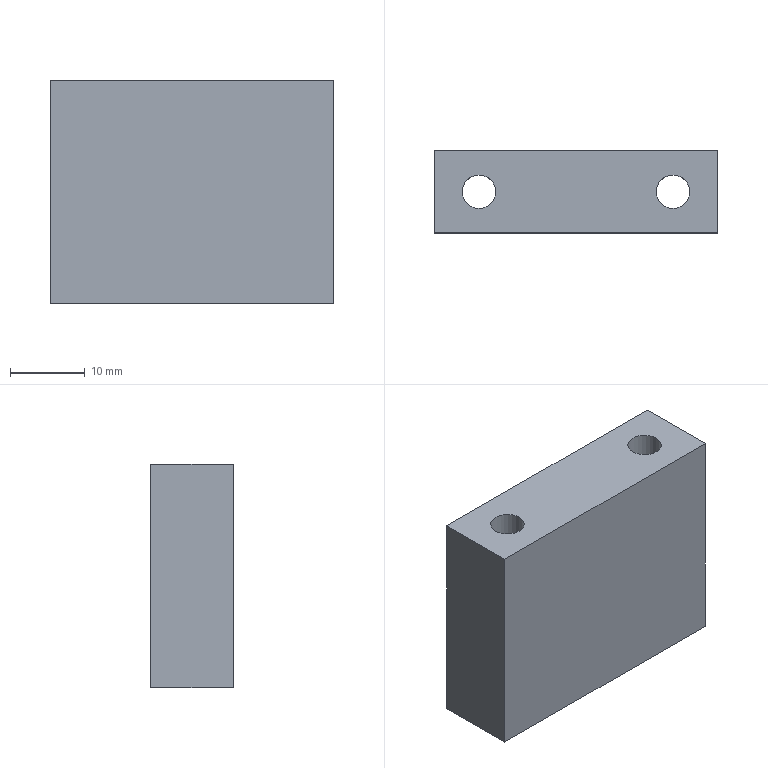Part | STEP file | 1 solid | 14 faces | box 38 x 11 x 30 mm | volume 9809 mm3 | plane 9 | cylinder 5 | commonest cylinder face diameters 8 x3 4.5 x2
STEP:
#1=CARTESIAN_POINT('',(0.,0.,0.));
#2=DIRECTION('',(0.,0.,1.));
#3=DIRECTION('',(1.,0.,0.));
#4=AXIS2_PLACEMENT_3D('',#1,#2,#3);
#5=CARTESIAN_POINT('',(-19.,5.5,-15.));
#6=VERTEX_POINT('',#5);
#7=CARTESIAN_POINT('',(19.,5.5,-15.));
#8=VERTEX_POINT('',#7);
#9=CARTESIAN_POINT('',(0.,5.5,-15.));
#10=DIRECTION('',(1.,0.,0.));
#11=VECTOR('',#10,1.);
#12=LINE('',#9,#11);
#13=CARTESIAN_POINT('',(0.,5.5,0.));
#14=DIRECTION('',(0.,-1.,0.));
#15=DIRECTION('',(0.,0.,-1.));
#16=AXIS2_PLACEMENT_3D('',#13,#14,#15);
#17=PLANE('',#16);
#18=CARTESIAN_POINT('',(15.,0.));
#19=DIRECTION('',(0.,1.));
#20=VECTOR('',#19,1.);
#21=LINE('',#18,#20);
#22=(GEOMETRIC_REPRESENTATION_CONTEXT(2)PARAMETRIC_REPRESENTATION_CONTEXT()REPRESENTATION_CONTEXT('',''));
#23=DEFINITIONAL_REPRESENTATION('',(#21),#22);
#24=PCURVE('',#17,#23);
#25=CARTESIAN_POINT('',(-19.,5.5,-15.));
#26=DIRECTION('',(0.,0.,1.));
#27=DIRECTION('',(1.,0.,0.));
#28=AXIS2_PLACEMENT_3D('',#25,#26,#27);
#29=PLANE('',#28);
#30=CARTESIAN_POINT('',(19.,0.));
#31=DIRECTION('',(1.,0.));
#32=VECTOR('',#31,1.);
#33=LINE('',#30,#32);
#34=(GEOMETRIC_REPRESENTATION_CONTEXT(2)PARAMETRIC_REPRESENTATION_CONTEXT()REPRESENTATION_CONTEXT('',''));
#35=DEFINITIONAL_REPRESENTATION('',(#33),#34);
#36=PCURVE('',#29,#35);
#37=SURFACE_CURVE('',#12,(#24,#36),.PCURVE_S1.);
#38=EDGE_CURVE('',#6,#8,#37,.T.);
#39=ORIENTED_EDGE('',*,*,#38,.F.);
#40=CARTESIAN_POINT('',(-19.,5.5,15.));
#41=VERTEX_POINT('',#40);
#42=CARTESIAN_POINT('',(-19.,5.5,0.));
#43=DIRECTION('',(0.,0.,-1.));
#44=VECTOR('',#43,1.);
#45=LINE('',#42,#44);
#46=CARTESIAN_POINT('',(0.,-19.));
#47=DIRECTION('',(1.,0.));
#48=VECTOR('',#47,1.);
#49=LINE('',#46,#48);
#50=(GEOMETRIC_REPRESENTATION_CONTEXT(2)PARAMETRIC_REPRESENTATION_CONTEXT()REPRESENTATION_CONTEXT('',''));
#51=DEFINITIONAL_REPRESENTATION('',(#49),#50);
#52=PCURVE('',#17,#51);
#53=CARTESIAN_POINT('',(-19.,5.5,15.));
#54=DIRECTION('',(1.,0.,0.));
#55=DIRECTION('',(0.,0.,-1.));
#56=AXIS2_PLACEMENT_3D('',#53,#54,#55);
#57=PLANE('',#56);
#58=CARTESIAN_POINT('',(15.,0.));
#59=DIRECTION('',(1.,0.));
#60=VECTOR('',#59,1.);
#61=LINE('',#58,#60);
#62=(GEOMETRIC_REPRESENTATION_CONTEXT(2)PARAMETRIC_REPRESENTATION_CONTEXT()REPRESENTATION_CONTEXT('',''));
#63=DEFINITIONAL_REPRESENTATION('',(#61),#62);
#64=PCURVE('',#57,#63);
#65=SURFACE_CURVE('',#45,(#52,#64),.PCURVE_S1.);
#66=EDGE_CURVE('',#41,#6,#65,.T.);
#67=ORIENTED_EDGE('',*,*,#66,.F.);
#68=CARTESIAN_POINT('',(19.,5.5,15.));
#69=VERTEX_POINT('',#68);
#70=CARTESIAN_POINT('',(0.,5.5,15.));
#71=DIRECTION('',(-1.,0.,0.));
#72=VECTOR('',#71,1.);
#73=LINE('',#70,#72);
#74=CARTESIAN_POINT('',(-15.,0.));
#75=DIRECTION('',(0.,-1.));
#76=VECTOR('',#75,1.);
#77=LINE('',#74,#76);
#78=(GEOMETRIC_REPRESENTATION_CONTEXT(2)PARAMETRIC_REPRESENTATION_CONTEXT()REPRESENTATION_CONTEXT('',''));
#79=DEFINITIONAL_REPRESENTATION('',(#77),#78);
#80=PCURVE('',#17,#79);
#81=CARTESIAN_POINT('',(-19.,5.5,15.));
#82=DIRECTION('',(0.,0.,-1.));
#83=DIRECTION('',(-1.,0.,0.));
#84=AXIS2_PLACEMENT_3D('',#81,#82,#83);
#85=PLANE('',#84);
#86=CARTESIAN_POINT('',(-19.,0.));
#87=DIRECTION('',(1.,0.));
#88=VECTOR('',#87,1.);
#89=LINE('',#86,#88);
#90=(GEOMETRIC_REPRESENTATION_CONTEXT(2)PARAMETRIC_REPRESENTATION_CONTEXT()REPRESENTATION_CONTEXT('',''));
#91=DEFINITIONAL_REPRESENTATION('',(#89),#90);
#92=PCURVE('',#85,#91);
#93=SURFACE_CURVE('',#73,(#80,#92),.PCURVE_S1.);
#94=EDGE_CURVE('',#69,#41,#93,.T.);
#95=ORIENTED_EDGE('',*,*,#94,.F.);
#96=CARTESIAN_POINT('',(19.,5.5,0.));
#97=DIRECTION('',(0.,0.,1.));
#98=VECTOR('',#97,1.);
#99=LINE('',#96,#98);
#100=CARTESIAN_POINT('',(0.,19.));
#101=DIRECTION('',(-1.,0.));
#102=VECTOR('',#101,1.);
#103=LINE('',#100,#102);
#104=(GEOMETRIC_REPRESENTATION_CONTEXT(2)PARAMETRIC_REPRESENTATION_CONTEXT()REPRESENTATION_CONTEXT('',''));
#105=DEFINITIONAL_REPRESENTATION('',(#103),#104);
#106=PCURVE('',#17,#105);
#107=CARTESIAN_POINT('',(19.,5.5,15.));
#108=DIRECTION('',(-1.,0.,0.));
#109=DIRECTION('',(0.,0.,1.));
#110=AXIS2_PLACEMENT_3D('',#107,#108,#109);
#111=PLANE('',#110);
#112=CARTESIAN_POINT('',(-15.,0.));
#113=DIRECTION('',(1.,0.));
#114=VECTOR('',#113,1.);
#115=LINE('',#112,#114);
#116=(GEOMETRIC_REPRESENTATION_CONTEXT(2)PARAMETRIC_REPRESENTATION_CONTEXT()REPRESENTATION_CONTEXT('',''));
#117=DEFINITIONAL_REPRESENTATION('',(#115),#116);
#118=PCURVE('',#111,#117);
#119=SURFACE_CURVE('',#99,(#106,#118),.PCURVE_S1.);
#120=EDGE_CURVE('',#8,#69,#119,.T.);
#121=ORIENTED_EDGE('',*,*,#120,.F.);
#122=EDGE_LOOP('',(#39,#67,#95,#121));
#123=FACE_BOUND('',#122,.T.);
#124=ADVANCED_FACE('',(#123),#17,.F.);
#125=CARTESIAN_POINT('',(19.,-5.5,-15.));
#126=VERTEX_POINT('',#125);
#127=CARTESIAN_POINT('',(19.,5.5,-15.));
#128=DIRECTION('',(0.,-1.,0.));
#129=VECTOR('',#128,1.);
#130=LINE('',#127,#129);
#131=CARTESIAN_POINT('',(-30.,0.));
#132=DIRECTION('',(0.,-1.));
#133=VECTOR('',#132,1.);
#134=LINE('',#131,#133);
#135=(GEOMETRIC_REPRESENTATION_CONTEXT(2)PARAMETRIC_REPRESENTATION_CONTEXT()REPRESENTATION_CONTEXT('',''));
#136=DEFINITIONAL_REPRESENTATION('',(#134),#135);
#137=PCURVE('',#111,#136);
#138=CARTESIAN_POINT('',(38.,0.));
#139=DIRECTION('',(0.,-1.));
#140=VECTOR('',#139,1.);
#141=LINE('',#138,#140);
#142=(GEOMETRIC_REPRESENTATION_CONTEXT(2)PARAMETRIC_REPRESENTATION_CONTEXT()REPRESENTATION_CONTEXT('',''));
#143=DEFINITIONAL_REPRESENTATION('',(#141),#142);
#144=PCURVE('',#29,#143);
#145=SURFACE_CURVE('',#130,(#137,#144),.PCURVE_S1.);
#146=EDGE_CURVE('',#8,#126,#145,.T.);
#147=ORIENTED_EDGE('',*,*,#146,.F.);
#148=ORIENTED_EDGE('',*,*,#120,.T.);
#149=CARTESIAN_POINT('',(19.,-5.5,15.));
#150=VERTEX_POINT('',#149);
#151=CARTESIAN_POINT('',(19.,5.5,15.));
#152=DIRECTION('',(0.,1.,0.));
#153=VECTOR('',#152,1.);
#154=LINE('',#151,#153);
#155=CARTESIAN_POINT('',(0.,0.));
#156=DIRECTION('',(0.,1.));
#157=VECTOR('',#156,1.);
#158=LINE('',#155,#157);
#159=(GEOMETRIC_REPRESENTATION_CONTEXT(2)PARAMETRIC_REPRESENTATION_CONTEXT()REPRESENTATION_CONTEXT('',''));
#160=DEFINITIONAL_REPRESENTATION('',(#158),#159);
#161=PCURVE('',#111,#160);
#162=CARTESIAN_POINT('',(-38.,0.));
#163=DIRECTION('',(0.,1.));
#164=VECTOR('',#163,1.);
#165=LINE('',#162,#164);
#166=(GEOMETRIC_REPRESENTATION_CONTEXT(2)PARAMETRIC_REPRESENTATION_CONTEXT()REPRESENTATION_CONTEXT('',''));
#167=DEFINITIONAL_REPRESENTATION('',(#165),#166);
#168=PCURVE('',#85,#167);
#169=SURFACE_CURVE('',#154,(#161,#168),.PCURVE_S1.);
#170=EDGE_CURVE('',#150,#69,#169,.T.);
#171=ORIENTED_EDGE('',*,*,#170,.F.);
#172=CARTESIAN_POINT('',(19.,-5.5,15.));
#173=DIRECTION('',(0.,0.,1.));
#174=VECTOR('',#173,1.);
#175=LINE('',#172,#174);
#176=CARTESIAN_POINT('',(0.,-11.));
#177=DIRECTION('',(1.,0.));
#178=VECTOR('',#177,1.);
#179=LINE('',#176,#178);
#180=(GEOMETRIC_REPRESENTATION_CONTEXT(2)PARAMETRIC_REPRESENTATION_CONTEXT()REPRESENTATION_CONTEXT('',''));
#181=DEFINITIONAL_REPRESENTATION('',(#179),#180);
#182=PCURVE('',#111,#181);
#183=CARTESIAN_POINT('',(0.,-5.5,0.));
#184=DIRECTION('',(0.,-1.,0.));
#185=DIRECTION('',(0.,0.,-1.));
#186=AXIS2_PLACEMENT_3D('',#183,#184,#185);
#187=PLANE('',#186);
#188=CARTESIAN_POINT('',(-15.,19.));
#189=DIRECTION('',(-1.,0.));
#190=VECTOR('',#189,1.);
#191=LINE('',#188,#190);
#192=(GEOMETRIC_REPRESENTATION_CONTEXT(2)PARAMETRIC_REPRESENTATION_CONTEXT()REPRESENTATION_CONTEXT('',''));
#193=DEFINITIONAL_REPRESENTATION('',(#191),#192);
#194=PCURVE('',#187,#193);
#195=SURFACE_CURVE('',#175,(#182,#194),.PCURVE_S1.);
#196=EDGE_CURVE('',#126,#150,#195,.T.);
#197=ORIENTED_EDGE('',*,*,#196,.F.);
#198=EDGE_LOOP('',(#147,#148,#171,#197));
#199=FACE_BOUND('',#198,.T.);
#200=ADVANCED_FACE('',(#199),#111,.F.);
#201=CARTESIAN_POINT('',(-17.,0.,-15.));
#202=VERTEX_POINT('',#201);
#203=CARTESIAN_POINT('',(-13.,0.,-15.));
#204=DIRECTION('',(0.,0.,-1.));
#205=DIRECTION('',(-1.,0.,0.));
#206=AXIS2_PLACEMENT_3D('',#203,#204,#205);
#207=CIRCLE('',#206,4.);
#208=CARTESIAN_POINT('',(2.,-5.5));
#209=CARTESIAN_POINT('',(2.,1.428));
#210=CARTESIAN_POINT('',(8.,-2.036));
#211=CARTESIAN_POINT('',(14.,-5.5));
#212=CARTESIAN_POINT('',(8.,-8.964));
#213=CARTESIAN_POINT('',(2.,-12.428));
#214=CARTESIAN_POINT('',(2.,-5.5));
#215=(BOUNDED_CURVE()B_SPLINE_CURVE(2,(#208,#209,#210,#211,#212,#213,#214),.UNSPECIFIED.,.T.,.F.)B_SPLINE_CURVE_WITH_KNOTS((1,2,2,2,2,1),(-2.094,0.,2.094,4.189,6.283,8.378),.UNSPECIFIED.)CURVE()GEOMETRIC_REPRESENTATION_ITEM()RATIONAL_B_SPLINE_CURVE((1.,0.5,1.,0.5,1.,0.5,1.))REPRESENTATION_ITEM(''));
#216=(GEOMETRIC_REPRESENTATION_CONTEXT(2)PARAMETRIC_REPRESENTATION_CONTEXT()REPRESENTATION_CONTEXT('',''));
#217=DEFINITIONAL_REPRESENTATION('',(#215),#216);
#218=PCURVE('',#29,#217);
#219=CARTESIAN_POINT('',(-13.,0.,-15.));
#220=DIRECTION('',(0.,0.,-1.));
#221=DIRECTION('',(-1.,0.,0.));
#222=AXIS2_PLACEMENT_3D('',#219,#220,#221);
#223=CYLINDRICAL_SURFACE('',#222,4.);
#224=CARTESIAN_POINT('',(0.,0.));
#225=DIRECTION('',(1.,0.));
#226=VECTOR('',#225,1.);
#227=LINE('',#224,#226);
#228=(GEOMETRIC_REPRESENTATION_CONTEXT(2)PARAMETRIC_REPRESENTATION_CONTEXT()REPRESENTATION_CONTEXT('',''));
#229=DEFINITIONAL_REPRESENTATION('',(#227),#228);
#230=PCURVE('',#223,#229);
#231=SURFACE_CURVE('',#207,(#218,#230),.PCURVE_S1.);
#232=EDGE_CURVE('',#202,#202,#231,.T.);
#233=ORIENTED_EDGE('',*,*,#232,.F.);
#234=EDGE_LOOP('',(#233));
#235=FACE_BOUND('',#234,.T.);
#236=CARTESIAN_POINT('',(9.,0.,-15.));
#237=VERTEX_POINT('',#236);
#238=CARTESIAN_POINT('',(13.,0.,-15.));
#239=DIRECTION('',(0.,0.,-1.));
#240=DIRECTION('',(-1.,0.,0.));
#241=AXIS2_PLACEMENT_3D('',#238,#239,#240);
#242=CIRCLE('',#241,4.);
#243=CARTESIAN_POINT('',(28.,-5.5));
#244=CARTESIAN_POINT('',(28.,1.428));
#245=CARTESIAN_POINT('',(34.,-2.036));
#246=CARTESIAN_POINT('',(40.,-5.5));
#247=CARTESIAN_POINT('',(34.,-8.964));
#248=CARTESIAN_POINT('',(28.,-12.428));
#249=CARTESIAN_POINT('',(28.,-5.5));
#250=(BOUNDED_CURVE()B_SPLINE_CURVE(2,(#243,#244,#245,#246,#247,#248,#249),.UNSPECIFIED.,.T.,.F.)B_SPLINE_CURVE_WITH_KNOTS((1,2,2,2,2,1),(-2.094,0.,2.094,4.189,6.283,8.378),.UNSPECIFIED.)CURVE()GEOMETRIC_REPRESENTATION_ITEM()RATIONAL_B_SPLINE_CURVE((1.,0.5,1.,0.5,1.,0.5,1.))REPRESENTATION_ITEM(''));
#251=(GEOMETRIC_REPRESENTATION_CONTEXT(2)PARAMETRIC_REPRESENTATION_CONTEXT()REPRESENTATION_CONTEXT('',''));
#252=DEFINITIONAL_REPRESENTATION('',(#250),#251);
#253=PCURVE('',#29,#252);
#254=CARTESIAN_POINT('',(13.,0.,-15.));
#255=DIRECTION('',(0.,0.,-1.));
#256=DIRECTION('',(-1.,0.,0.));
#257=AXIS2_PLACEMENT_3D('',#254,#255,#256);
#258=CYLINDRICAL_SURFACE('',#257,4.);
#259=CARTESIAN_POINT('',(0.,0.));
#260=DIRECTION('',(1.,0.));
#261=VECTOR('',#260,1.);
#262=LINE('',#259,#261);
#263=(GEOMETRIC_REPRESENTATION_CONTEXT(2)PARAMETRIC_REPRESENTATION_CONTEXT()REPRESENTATION_CONTEXT('',''));
#264=DEFINITIONAL_REPRESENTATION('',(#262),#263);
#265=PCURVE('',#258,#264);
#266=SURFACE_CURVE('',#242,(#253,#265),.PCURVE_S1.);
#267=EDGE_CURVE('',#237,#237,#266,.T.);
#268=ORIENTED_EDGE('',*,*,#267,.F.);
#269=EDGE_LOOP('',(#268));
#270=FACE_BOUND('',#269,.T.);
#271=CARTESIAN_POINT('',(-4.,0.,-15.));
#272=VERTEX_POINT('',#271);
#273=CARTESIAN_POINT('',(0.,0.,-15.));
#274=DIRECTION('',(0.,0.,-1.));
#275=DIRECTION('',(-1.,0.,0.));
#276=AXIS2_PLACEMENT_3D('',#273,#274,#275);
#277=CIRCLE('',#276,4.);
#278=CARTESIAN_POINT('',(15.,-5.5));
#279=CARTESIAN_POINT('',(15.,1.428));
#280=CARTESIAN_POINT('',(21.,-2.036));
#281=CARTESIAN_POINT('',(27.,-5.5));
#282=CARTESIAN_POINT('',(21.,-8.964));
#283=CARTESIAN_POINT('',(15.,-12.428));
#284=CARTESIAN_POINT('',(15.,-5.5));
#285=(BOUNDED_CURVE()B_SPLINE_CURVE(2,(#278,#279,#280,#281,#282,#283,#284),.UNSPECIFIED.,.T.,.F.)B_SPLINE_CURVE_WITH_KNOTS((1,2,2,2,2,1),(-2.094,0.,2.094,4.189,6.283,8.378),.UNSPECIFIED.)CURVE()GEOMETRIC_REPRESENTATION_ITEM()RATIONAL_B_SPLINE_CURVE((1.,0.5,1.,0.5,1.,0.5,1.))REPRESENTATION_ITEM(''));
#286=(GEOMETRIC_REPRESENTATION_CONTEXT(2)PARAMETRIC_REPRESENTATION_CONTEXT()REPRESENTATION_CONTEXT('',''));
#287=DEFINITIONAL_REPRESENTATION('',(#285),#286);
#288=PCURVE('',#29,#287);
#289=CARTESIAN_POINT('',(0.,0.,-7.));
#290=DIRECTION('',(0.,0.,-1.));
#291=DIRECTION('',(-1.,0.,0.));
#292=AXIS2_PLACEMENT_3D('',#289,#290,#291);
#293=CYLINDRICAL_SURFACE('',#292,4.);
#294=CARTESIAN_POINT('',(0.,8.));
#295=DIRECTION('',(1.,0.));
#296=VECTOR('',#295,1.);
#297=LINE('',#294,#296);
#298=(GEOMETRIC_REPRESENTATION_CONTEXT(2)PARAMETRIC_REPRESENTATION_CONTEXT()REPRESENTATION_CONTEXT('',''));
#299=DEFINITIONAL_REPRESENTATION('',(#297),#298);
#300=PCURVE('',#293,#299);
#301=SURFACE_CURVE('',#277,(#288,#300),.PCURVE_S1.);
#302=EDGE_CURVE('',#272,#272,#301,.T.);
#303=ORIENTED_EDGE('',*,*,#302,.F.);
#304=EDGE_LOOP('',(#303));
#305=FACE_BOUND('',#304,.T.);
#306=CARTESIAN_POINT('',(-19.,-5.5,-15.));
#307=VERTEX_POINT('',#306);
#308=CARTESIAN_POINT('',(-19.,5.5,-15.));
#309=DIRECTION('',(0.,-1.,0.));
#310=VECTOR('',#309,1.);
#311=LINE('',#308,#310);
#312=CARTESIAN_POINT('',(0.,0.));
#313=DIRECTION('',(0.,-1.));
#314=VECTOR('',#313,1.);
#315=LINE('',#312,#314);
#316=(GEOMETRIC_REPRESENTATION_CONTEXT(2)PARAMETRIC_REPRESENTATION_CONTEXT()REPRESENTATION_CONTEXT('',''));
#317=DEFINITIONAL_REPRESENTATION('',(#315),#316);
#318=PCURVE('',#29,#317);
#319=CARTESIAN_POINT('',(30.,0.));
#320=DIRECTION('',(0.,-1.));
#321=VECTOR('',#320,1.);
#322=LINE('',#319,#321);
#323=(GEOMETRIC_REPRESENTATION_CONTEXT(2)PARAMETRIC_REPRESENTATION_CONTEXT()REPRESENTATION_CONTEXT('',''));
#324=DEFINITIONAL_REPRESENTATION('',(#322),#323);
#325=PCURVE('',#57,#324);
#326=SURFACE_CURVE('',#311,(#318,#325),.PCURVE_S1.);
#327=EDGE_CURVE('',#6,#307,#326,.T.);
#328=ORIENTED_EDGE('',*,*,#327,.F.);
#329=ORIENTED_EDGE('',*,*,#38,.T.);
#330=ORIENTED_EDGE('',*,*,#146,.T.);
#331=CARTESIAN_POINT('',(-19.,-5.5,-15.));
#332=DIRECTION('',(1.,0.,0.));
#333=VECTOR('',#332,1.);
#334=LINE('',#331,#333);
#335=CARTESIAN_POINT('',(0.,-11.));
#336=DIRECTION('',(1.,0.));
#337=VECTOR('',#336,1.);
#338=LINE('',#335,#337);
#339=(GEOMETRIC_REPRESENTATION_CONTEXT(2)PARAMETRIC_REPRESENTATION_CONTEXT()REPRESENTATION_CONTEXT('',''));
#340=DEFINITIONAL_REPRESENTATION('',(#338),#339);
#341=PCURVE('',#29,#340);
#342=CARTESIAN_POINT('',(15.,-19.));
#343=DIRECTION('',(0.,1.));
#344=VECTOR('',#343,1.);
#345=LINE('',#342,#344);
#346=(GEOMETRIC_REPRESENTATION_CONTEXT(2)PARAMETRIC_REPRESENTATION_CONTEXT()REPRESENTATION_CONTEXT('',''));
#347=DEFINITIONAL_REPRESENTATION('',(#345),#346);
#348=PCURVE('',#187,#347);
#349=SURFACE_CURVE('',#334,(#341,#348),.PCURVE_S1.);
#350=EDGE_CURVE('',#307,#126,#349,.T.);
#351=ORIENTED_EDGE('',*,*,#350,.F.);
#352=EDGE_LOOP('',(#328,#329,#330,#351));
#353=FACE_BOUND('',#352,.T.);
#354=ADVANCED_FACE('',(#235,#270,#305,#353),#29,.F.);
#355=CARTESIAN_POINT('',(-19.,-5.5,15.));
#356=VERTEX_POINT('',#355);
#357=CARTESIAN_POINT('',(-19.,5.5,15.));
#358=DIRECTION('',(0.,-1.,0.));
#359=VECTOR('',#358,1.);
#360=LINE('',#357,#359);
#361=CARTESIAN_POINT('',(0.,0.));
#362=DIRECTION('',(0.,-1.));
#363=VECTOR('',#362,1.);
#364=LINE('',#361,#363);
#365=(GEOMETRIC_REPRESENTATION_CONTEXT(2)PARAMETRIC_REPRESENTATION_CONTEXT()REPRESENTATION_CONTEXT('',''));
#366=DEFINITIONAL_REPRESENTATION('',(#364),#365);
#367=PCURVE('',#57,#366);
#368=CARTESIAN_POINT('',(0.,0.));
#369=DIRECTION('',(0.,-1.));
#370=VECTOR('',#369,1.);
#371=LINE('',#368,#370);
#372=(GEOMETRIC_REPRESENTATION_CONTEXT(2)PARAMETRIC_REPRESENTATION_CONTEXT()REPRESENTATION_CONTEXT('',''));
#373=DEFINITIONAL_REPRESENTATION('',(#371),#372);
#374=PCURVE('',#85,#373);
#375=SURFACE_CURVE('',#360,(#367,#374),.PCURVE_S1.);
#376=EDGE_CURVE('',#41,#356,#375,.T.);
#377=ORIENTED_EDGE('',*,*,#376,.F.);
#378=ORIENTED_EDGE('',*,*,#66,.T.);
#379=ORIENTED_EDGE('',*,*,#327,.T.);
#380=CARTESIAN_POINT('',(-19.,-5.5,15.));
#381=DIRECTION('',(0.,0.,-1.));
#382=VECTOR('',#381,1.);
#383=LINE('',#380,#382);
#384=CARTESIAN_POINT('',(0.,-11.));
#385=DIRECTION('',(1.,0.));
#386=VECTOR('',#385,1.);
#387=LINE('',#384,#386);
#388=(GEOMETRIC_REPRESENTATION_CONTEXT(2)PARAMETRIC_REPRESENTATION_CONTEXT()REPRESENTATION_CONTEXT('',''));
#389=DEFINITIONAL_REPRESENTATION('',(#387),#388);
#390=PCURVE('',#57,#389);
#391=CARTESIAN_POINT('',(-15.,-19.));
#392=DIRECTION('',(1.,0.));
#393=VECTOR('',#392,1.);
#394=LINE('',#391,#393);
#395=(GEOMETRIC_REPRESENTATION_CONTEXT(2)PARAMETRIC_REPRESENTATION_CONTEXT()REPRESENTATION_CONTEXT('',''));
#396=DEFINITIONAL_REPRESENTATION('',(#394),#395);
#397=PCURVE('',#187,#396);
#398=SURFACE_CURVE('',#383,(#390,#397),.PCURVE_S1.);
#399=EDGE_CURVE('',#356,#307,#398,.T.);
#400=ORIENTED_EDGE('',*,*,#399,.F.);
#401=EDGE_LOOP('',(#377,#378,#379,#400));
#402=FACE_BOUND('',#401,.T.);
#403=ADVANCED_FACE('',(#402),#57,.F.);
#404=CARTESIAN_POINT('',(-15.25,0.,15.));
#405=VERTEX_POINT('',#404);
#406=CARTESIAN_POINT('',(-13.,0.,15.));
#407=DIRECTION('',(0.,0.,1.));
#408=DIRECTION('',(-1.,0.,0.));
#409=AXIS2_PLACEMENT_3D('',#406,#407,#408);
#410=CIRCLE('',#409,2.25);
#411=CARTESIAN_POINT('',(-3.75,-5.5));
#412=CARTESIAN_POINT('',(-3.75,-9.397));
#413=CARTESIAN_POINT('',(-7.125,-7.449));
#414=CARTESIAN_POINT('',(-10.5,-5.5));
#415=CARTESIAN_POINT('',(-7.125,-3.551));
#416=CARTESIAN_POINT('',(-3.75,-1.603));
#417=CARTESIAN_POINT('',(-3.75,-5.5));
#418=(BOUNDED_CURVE()B_SPLINE_CURVE(2,(#411,#412,#413,#414,#415,#416,#417),.UNSPECIFIED.,.T.,.F.)B_SPLINE_CURVE_WITH_KNOTS((1,2,2,2,2,1),(-2.094,0.,2.094,4.189,6.283,8.378),.UNSPECIFIED.)CURVE()GEOMETRIC_REPRESENTATION_ITEM()RATIONAL_B_SPLINE_CURVE((1.,0.5,1.,0.5,1.,0.5,1.))REPRESENTATION_ITEM(''));
#419=(GEOMETRIC_REPRESENTATION_CONTEXT(2)PARAMETRIC_REPRESENTATION_CONTEXT()REPRESENTATION_CONTEXT('',''));
#420=DEFINITIONAL_REPRESENTATION('',(#418),#419);
#421=PCURVE('',#85,#420);
#422=CARTESIAN_POINT('',(-13.,0.,-15.));
#423=DIRECTION('',(0.,0.,-1.));
#424=DIRECTION('',(-1.,0.,0.));
#425=AXIS2_PLACEMENT_3D('',#422,#423,#424);
#426=CYLINDRICAL_SURFACE('',#425,2.25);
#427=CARTESIAN_POINT('',(6.283,-30.));
#428=DIRECTION('',(-1.,0.));
#429=VECTOR('',#428,1.);
#430=LINE('',#427,#429);
#431=(GEOMETRIC_REPRESENTATION_CONTEXT(2)PARAMETRIC_REPRESENTATION_CONTEXT()REPRESENTATION_CONTEXT('',''));
#432=DEFINITIONAL_REPRESENTATION('',(#430),#431);
#433=PCURVE('',#426,#432);
#434=SURFACE_CURVE('',#410,(#421,#433),.PCURVE_S1.);
#435=EDGE_CURVE('',#405,#405,#434,.T.);
#436=ORIENTED_EDGE('',*,*,#435,.F.);
#437=EDGE_LOOP('',(#436));
#438=FACE_BOUND('',#437,.T.);
#439=CARTESIAN_POINT('',(10.75,0.,15.));
#440=VERTEX_POINT('',#439);
#441=CARTESIAN_POINT('',(13.,0.,15.));
#442=DIRECTION('',(0.,0.,1.));
#443=DIRECTION('',(-1.,0.,0.));
#444=AXIS2_PLACEMENT_3D('',#441,#442,#443);
#445=CIRCLE('',#444,2.25);
#446=CARTESIAN_POINT('',(-29.75,-5.5));
#447=CARTESIAN_POINT('',(-29.75,-9.397));
#448=CARTESIAN_POINT('',(-33.125,-7.449));
#449=CARTESIAN_POINT('',(-36.5,-5.5));
#450=CARTESIAN_POINT('',(-33.125,-3.551));
#451=CARTESIAN_POINT('',(-29.75,-1.603));
#452=CARTESIAN_POINT('',(-29.75,-5.5));
#453=(BOUNDED_CURVE()B_SPLINE_CURVE(2,(#446,#447,#448,#449,#450,#451,#452),.UNSPECIFIED.,.T.,.F.)B_SPLINE_CURVE_WITH_KNOTS((1,2,2,2,2,1),(-2.094,0.,2.094,4.189,6.283,8.378),.UNSPECIFIED.)CURVE()GEOMETRIC_REPRESENTATION_ITEM()RATIONAL_B_SPLINE_CURVE((1.,0.5,1.,0.5,1.,0.5,1.))REPRESENTATION_ITEM(''));
#454=(GEOMETRIC_REPRESENTATION_CONTEXT(2)PARAMETRIC_REPRESENTATION_CONTEXT()REPRESENTATION_CONTEXT('',''));
#455=DEFINITIONAL_REPRESENTATION('',(#453),#454);
#456=PCURVE('',#85,#455);
#457=CARTESIAN_POINT('',(13.,0.,-15.));
#458=DIRECTION('',(0.,0.,-1.));
#459=DIRECTION('',(-1.,0.,0.));
#460=AXIS2_PLACEMENT_3D('',#457,#458,#459);
#461=CYLINDRICAL_SURFACE('',#460,2.25);
#462=CARTESIAN_POINT('',(6.283,-30.));
#463=DIRECTION('',(-1.,0.));
#464=VECTOR('',#463,1.);
#465=LINE('',#462,#464);
#466=(GEOMETRIC_REPRESENTATION_CONTEXT(2)PARAMETRIC_REPRESENTATION_CONTEXT()REPRESENTATION_CONTEXT('',''));
#467=DEFINITIONAL_REPRESENTATION('',(#465),#466);
#468=PCURVE('',#461,#467);
#469=SURFACE_CURVE('',#445,(#456,#468),.PCURVE_S1.);
#470=EDGE_CURVE('',#440,#440,#469,.T.);
#471=ORIENTED_EDGE('',*,*,#470,.F.);
#472=EDGE_LOOP('',(#471));
#473=FACE_BOUND('',#472,.T.);
#474=ORIENTED_EDGE('',*,*,#170,.T.);
#475=ORIENTED_EDGE('',*,*,#94,.T.);
#476=ORIENTED_EDGE('',*,*,#376,.T.);
#477=CARTESIAN_POINT('',(-19.,-5.5,15.));
#478=DIRECTION('',(-1.,0.,0.));
#479=VECTOR('',#478,1.);
#480=LINE('',#477,#479);
#481=CARTESIAN_POINT('',(0.,-11.));
#482=DIRECTION('',(1.,0.));
#483=VECTOR('',#482,1.);
#484=LINE('',#481,#483);
#485=(GEOMETRIC_REPRESENTATION_CONTEXT(2)PARAMETRIC_REPRESENTATION_CONTEXT()REPRESENTATION_CONTEXT('',''));
#486=DEFINITIONAL_REPRESENTATION('',(#484),#485);
#487=PCURVE('',#85,#486);
#488=CARTESIAN_POINT('',(-15.,-19.));
#489=DIRECTION('',(0.,-1.));
#490=VECTOR('',#489,1.);
#491=LINE('',#488,#490);
#492=(GEOMETRIC_REPRESENTATION_CONTEXT(2)PARAMETRIC_REPRESENTATION_CONTEXT()REPRESENTATION_CONTEXT('',''));
#493=DEFINITIONAL_REPRESENTATION('',(#491),#492);
#494=PCURVE('',#187,#493);
#495=SURFACE_CURVE('',#480,(#487,#494),.PCURVE_S1.);
#496=EDGE_CURVE('',#150,#356,#495,.T.);
#497=ORIENTED_EDGE('',*,*,#496,.F.);
#498=EDGE_LOOP('',(#474,#475,#476,#497));
#499=FACE_BOUND('',#498,.T.);
#500=ADVANCED_FACE('',(#438,#473,#499),#85,.F.);
#501=ORIENTED_EDGE('',*,*,#399,.T.);
#502=ORIENTED_EDGE('',*,*,#350,.T.);
#503=ORIENTED_EDGE('',*,*,#196,.T.);
#504=ORIENTED_EDGE('',*,*,#496,.T.);
#505=EDGE_LOOP('',(#501,#502,#503,#504));
#506=FACE_BOUND('',#505,.T.);
#507=ADVANCED_FACE('',(#506),#187,.T.);
#508=CARTESIAN_POINT('',(-17.,0.,5.));
#509=VERTEX_POINT('',#508);
#510=CARTESIAN_POINT('',(-13.,0.,5.));
#511=DIRECTION('',(0.,0.,-1.));
#512=DIRECTION('',(-1.,0.,0.));
#513=AXIS2_PLACEMENT_3D('',#510,#511,#512);
#514=CIRCLE('',#513,4.);
#515=CARTESIAN_POINT('',(0.,-20.));
#516=DIRECTION('',(1.,0.));
#517=VECTOR('',#516,1.);
#518=LINE('',#515,#517);
#519=(GEOMETRIC_REPRESENTATION_CONTEXT(2)PARAMETRIC_REPRESENTATION_CONTEXT()REPRESENTATION_CONTEXT('',''));
#520=DEFINITIONAL_REPRESENTATION('',(#518),#519);
#521=PCURVE('',#223,#520);
#522=CARTESIAN_POINT('',(-10.75,0.,5.));
#523=DIRECTION('',(0.,0.,1.));
#524=DIRECTION('',(1.,0.,0.));
#525=AXIS2_PLACEMENT_3D('',#522,#523,#524);
#526=PLANE('',#525);
#527=CARTESIAN_POINT('',(-6.25,0.));
#528=CARTESIAN_POINT('',(-6.25,6.928));
#529=CARTESIAN_POINT('',(-0.25,3.464));
#530=CARTESIAN_POINT('',(5.75,0.));
#531=CARTESIAN_POINT('',(-0.25,-3.464));
#532=CARTESIAN_POINT('',(-6.25,-6.928));
#533=CARTESIAN_POINT('',(-6.25,0.));
#534=(BOUNDED_CURVE()B_SPLINE_CURVE(2,(#527,#528,#529,#530,#531,#532,#533),.UNSPECIFIED.,.T.,.F.)B_SPLINE_CURVE_WITH_KNOTS((1,2,2,2,2,1),(-2.094,0.,2.094,4.189,6.283,8.378),.UNSPECIFIED.)CURVE()GEOMETRIC_REPRESENTATION_ITEM()RATIONAL_B_SPLINE_CURVE((1.,0.5,1.,0.5,1.,0.5,1.))REPRESENTATION_ITEM(''));
#535=(GEOMETRIC_REPRESENTATION_CONTEXT(2)PARAMETRIC_REPRESENTATION_CONTEXT()REPRESENTATION_CONTEXT('',''));
#536=DEFINITIONAL_REPRESENTATION('',(#534),#535);
#537=PCURVE('',#526,#536);
#538=SURFACE_CURVE('',#514,(#521,#537),.PCURVE_S1.);
#539=EDGE_CURVE('',#509,#509,#538,.T.);
#540=ORIENTED_EDGE('',*,*,#539,.T.);
#541=CARTESIAN_POINT('',(-17.,0.,5.));
#542=CARTESIAN_POINT('',(-17.,0.,-15.));
#543=B_SPLINE_CURVE_WITH_KNOTS('',1,(#541,#542),.UNSPECIFIED.,.F.,.F.,(2,2),(-20.,0.),.PIECEWISE_BEZIER_KNOTS.);
#544=CARTESIAN_POINT('',(6.283,0.));
#545=DIRECTION('',(0.,1.));
#546=VECTOR('',#545,1.);
#547=LINE('',#544,#546);
#548=(GEOMETRIC_REPRESENTATION_CONTEXT(2)PARAMETRIC_REPRESENTATION_CONTEXT()REPRESENTATION_CONTEXT('',''));
#549=DEFINITIONAL_REPRESENTATION('',(#547),#548);
#550=PCURVE('',#223,#549);
#551=CARTESIAN_POINT('',(0.,0.));
#552=DIRECTION('',(0.,1.));
#553=VECTOR('',#552,1.);
#554=LINE('',#551,#553);
#555=(GEOMETRIC_REPRESENTATION_CONTEXT(2)PARAMETRIC_REPRESENTATION_CONTEXT()REPRESENTATION_CONTEXT('',''));
#556=DEFINITIONAL_REPRESENTATION('',(#554),#555);
#557=PCURVE('',#223,#556);
#558=SEAM_CURVE('',#543,(#550,#557),.PCURVE_S1.);
#559=EDGE_CURVE('',#509,#202,#558,.T.);
#560=ORIENTED_EDGE('',*,*,#559,.T.);
#561=ORIENTED_EDGE('',*,*,#232,.F.);
#562=ORIENTED_EDGE('',*,*,#559,.F.);
#563=EDGE_LOOP('',(#540,#560,#561,#562));
#564=FACE_BOUND('',#563,.F.);
#565=ADVANCED_FACE('',(#564),#223,.F.);
#566=CARTESIAN_POINT('',(9.,0.,5.));
#567=VERTEX_POINT('',#566);
#568=CARTESIAN_POINT('',(13.,0.,5.));
#569=DIRECTION('',(0.,0.,-1.));
#570=DIRECTION('',(-1.,0.,0.));
#571=AXIS2_PLACEMENT_3D('',#568,#569,#570);
#572=CIRCLE('',#571,4.);
#573=CARTESIAN_POINT('',(0.,-20.));
#574=DIRECTION('',(1.,0.));
#575=VECTOR('',#574,1.);
#576=LINE('',#573,#575);
#577=(GEOMETRIC_REPRESENTATION_CONTEXT(2)PARAMETRIC_REPRESENTATION_CONTEXT()REPRESENTATION_CONTEXT('',''));
#578=DEFINITIONAL_REPRESENTATION('',(#576),#577);
#579=PCURVE('',#258,#578);
#580=CARTESIAN_POINT('',(15.25,0.,5.));
#581=DIRECTION('',(0.,0.,1.));
#582=DIRECTION('',(1.,0.,0.));
#583=AXIS2_PLACEMENT_3D('',#580,#581,#582);
#584=PLANE('',#583);
#585=CARTESIAN_POINT('',(-6.25,0.));
#586=CARTESIAN_POINT('',(-6.25,6.928));
#587=CARTESIAN_POINT('',(-0.25,3.464));
#588=CARTESIAN_POINT('',(5.75,0.));
#589=CARTESIAN_POINT('',(-0.25,-3.464));
#590=CARTESIAN_POINT('',(-6.25,-6.928));
#591=CARTESIAN_POINT('',(-6.25,0.));
#592=(BOUNDED_CURVE()B_SPLINE_CURVE(2,(#585,#586,#587,#588,#589,#590,#591),.UNSPECIFIED.,.T.,.F.)B_SPLINE_CURVE_WITH_KNOTS((1,2,2,2,2,1),(-2.094,0.,2.094,4.189,6.283,8.378),.UNSPECIFIED.)CURVE()GEOMETRIC_REPRESENTATION_ITEM()RATIONAL_B_SPLINE_CURVE((1.,0.5,1.,0.5,1.,0.5,1.))REPRESENTATION_ITEM(''));
#593=(GEOMETRIC_REPRESENTATION_CONTEXT(2)PARAMETRIC_REPRESENTATION_CONTEXT()REPRESENTATION_CONTEXT('',''));
#594=DEFINITIONAL_REPRESENTATION('',(#592),#593);
#595=PCURVE('',#584,#594);
#596=SURFACE_CURVE('',#572,(#579,#595),.PCURVE_S1.);
#597=EDGE_CURVE('',#567,#567,#596,.T.);
#598=ORIENTED_EDGE('',*,*,#597,.T.);
#599=CARTESIAN_POINT('',(9.,0.,5.));
#600=CARTESIAN_POINT('',(9.,0.,-15.));
#601=B_SPLINE_CURVE_WITH_KNOTS('',1,(#599,#600),.UNSPECIFIED.,.F.,.F.,(2,2),(-20.,0.),.PIECEWISE_BEZIER_KNOTS.);
#602=CARTESIAN_POINT('',(6.283,0.));
#603=DIRECTION('',(0.,1.));
#604=VECTOR('',#603,1.);
#605=LINE('',#602,#604);
#606=(GEOMETRIC_REPRESENTATION_CONTEXT(2)PARAMETRIC_REPRESENTATION_CONTEXT()REPRESENTATION_CONTEXT('',''));
#607=DEFINITIONAL_REPRESENTATION('',(#605),#606);
#608=PCURVE('',#258,#607);
#609=CARTESIAN_POINT('',(0.,0.));
#610=DIRECTION('',(0.,1.));
#611=VECTOR('',#610,1.);
#612=LINE('',#609,#611);
#613=(GEOMETRIC_REPRESENTATION_CONTEXT(2)PARAMETRIC_REPRESENTATION_CONTEXT()REPRESENTATION_CONTEXT('',''));
#614=DEFINITIONAL_REPRESENTATION('',(#612),#613);
#615=PCURVE('',#258,#614);
#616=SEAM_CURVE('',#601,(#608,#615),.PCURVE_S1.);
#617=EDGE_CURVE('',#567,#237,#616,.T.);
#618=ORIENTED_EDGE('',*,*,#617,.T.);
#619=ORIENTED_EDGE('',*,*,#267,.F.);
#620=ORIENTED_EDGE('',*,*,#617,.F.);
#621=EDGE_LOOP('',(#598,#618,#619,#620));
#622=FACE_BOUND('',#621,.F.);
#623=ADVANCED_FACE('',(#622),#258,.F.);
#624=CARTESIAN_POINT('',(-4.,0.,-7.));
#625=VERTEX_POINT('',#624);
#626=CARTESIAN_POINT('',(0.,0.,-7.));
#627=DIRECTION('',(0.,0.,-1.));
#628=DIRECTION('',(-1.,0.,0.));
#629=AXIS2_PLACEMENT_3D('',#626,#627,#628);
#630=CIRCLE('',#629,4.);
#631=CARTESIAN_POINT('',(0.,0.));
#632=DIRECTION('',(1.,0.));
#633=VECTOR('',#632,1.);
#634=LINE('',#631,#633);
#635=(GEOMETRIC_REPRESENTATION_CONTEXT(2)PARAMETRIC_REPRESENTATION_CONTEXT()REPRESENTATION_CONTEXT('',''));
#636=DEFINITIONAL_REPRESENTATION('',(#634),#635);
#637=PCURVE('',#293,#636);
#638=CARTESIAN_POINT('',(0.,0.,-7.));
#639=DIRECTION('',(0.,0.,-1.));
#640=DIRECTION('',(-1.,0.,0.));
#641=AXIS2_PLACEMENT_3D('',#638,#639,#640);
#642=PLANE('',#641);
#643=CARTESIAN_POINT('',(0.,0.));
#644=DIRECTION('',(1.,0.));
#645=AXIS2_PLACEMENT_2D('',#643,#644);
#646=CIRCLE('',#645,4.);
#647=(GEOMETRIC_REPRESENTATION_CONTEXT(2)PARAMETRIC_REPRESENTATION_CONTEXT()REPRESENTATION_CONTEXT('',''));
#648=DEFINITIONAL_REPRESENTATION('',(#646),#647);
#649=PCURVE('',#642,#648);
#650=SURFACE_CURVE('',#630,(#637,#649),.PCURVE_S1.);
#651=EDGE_CURVE('',#625,#625,#650,.T.);
#652=ORIENTED_EDGE('',*,*,#651,.T.);
#653=CARTESIAN_POINT('',(-4.,0.,-7.));
#654=CARTESIAN_POINT('',(-4.,0.,-15.));
#655=B_SPLINE_CURVE_WITH_KNOTS('',1,(#653,#654),.UNSPECIFIED.,.F.,.F.,(2,2),(0.,8.),.PIECEWISE_BEZIER_KNOTS.);
#656=CARTESIAN_POINT('',(6.283,0.));
#657=DIRECTION('',(0.,1.));
#658=VECTOR('',#657,1.);
#659=LINE('',#656,#658);
#660=(GEOMETRIC_REPRESENTATION_CONTEXT(2)PARAMETRIC_REPRESENTATION_CONTEXT()REPRESENTATION_CONTEXT('',''));
#661=DEFINITIONAL_REPRESENTATION('',(#659),#660);
#662=PCURVE('',#293,#661);
#663=CARTESIAN_POINT('',(0.,0.));
#664=DIRECTION('',(0.,1.));
#665=VECTOR('',#664,1.);
#666=LINE('',#663,#665);
#667=(GEOMETRIC_REPRESENTATION_CONTEXT(2)PARAMETRIC_REPRESENTATION_CONTEXT()REPRESENTATION_CONTEXT('',''));
#668=DEFINITIONAL_REPRESENTATION('',(#666),#667);
#669=PCURVE('',#293,#668);
#670=SEAM_CURVE('',#655,(#662,#669),.PCURVE_S1.);
#671=EDGE_CURVE('',#625,#272,#670,.T.);
#672=ORIENTED_EDGE('',*,*,#671,.T.);
#673=ORIENTED_EDGE('',*,*,#302,.F.);
#674=ORIENTED_EDGE('',*,*,#671,.F.);
#675=EDGE_LOOP('',(#652,#672,#673,#674));
#676=FACE_BOUND('',#675,.F.);
#677=ADVANCED_FACE('',(#676),#293,.F.);
#678=ORIENTED_EDGE('',*,*,#435,.F.);
#679=CARTESIAN_POINT('',(-15.25,0.,5.));
#680=VERTEX_POINT('',#679);
#681=CARTESIAN_POINT('',(-15.25,0.,15.));
#682=CARTESIAN_POINT('',(-15.25,0.,5.));
#683=B_SPLINE_CURVE_WITH_KNOTS('',1,(#681,#682),.UNSPECIFIED.,.F.,.F.,(2,2),(-30.,-20.),.PIECEWISE_BEZIER_KNOTS.);
#684=CARTESIAN_POINT('',(6.283,0.));
#685=DIRECTION('',(0.,1.));
#686=VECTOR('',#685,1.);
#687=LINE('',#684,#686);
#688=(GEOMETRIC_REPRESENTATION_CONTEXT(2)PARAMETRIC_REPRESENTATION_CONTEXT()REPRESENTATION_CONTEXT('',''));
#689=DEFINITIONAL_REPRESENTATION('',(#687),#688);
#690=PCURVE('',#426,#689);
#691=CARTESIAN_POINT('',(0.,0.));
#692=DIRECTION('',(0.,1.));
#693=VECTOR('',#692,1.);
#694=LINE('',#691,#693);
#695=(GEOMETRIC_REPRESENTATION_CONTEXT(2)PARAMETRIC_REPRESENTATION_CONTEXT()REPRESENTATION_CONTEXT('',''));
#696=DEFINITIONAL_REPRESENTATION('',(#694),#695);
#697=PCURVE('',#426,#696);
#698=SEAM_CURVE('',#683,(#690,#697),.PCURVE_S1.);
#699=EDGE_CURVE('',#405,#680,#698,.T.);
#700=ORIENTED_EDGE('',*,*,#699,.T.);
#701=CARTESIAN_POINT('',(-13.,0.,5.));
#702=DIRECTION('',(0.,0.,1.));
#703=DIRECTION('',(-1.,0.,0.));
#704=AXIS2_PLACEMENT_3D('',#701,#702,#703);
#705=CIRCLE('',#704,2.25);
#706=CARTESIAN_POINT('',(6.283,-20.));
#707=DIRECTION('',(-1.,0.));
#708=VECTOR('',#707,1.);
#709=LINE('',#706,#708);
#710=(GEOMETRIC_REPRESENTATION_CONTEXT(2)PARAMETRIC_REPRESENTATION_CONTEXT()REPRESENTATION_CONTEXT('',''));
#711=DEFINITIONAL_REPRESENTATION('',(#709),#710);
#712=PCURVE('',#426,#711);
#713=CARTESIAN_POINT('',(-2.25,0.));
#714=DIRECTION('',(-1.,0.));
#715=AXIS2_PLACEMENT_2D('',#713,#714);
#716=CIRCLE('',#715,2.25);
#717=(GEOMETRIC_REPRESENTATION_CONTEXT(2)PARAMETRIC_REPRESENTATION_CONTEXT()REPRESENTATION_CONTEXT('',''));
#718=DEFINITIONAL_REPRESENTATION('',(#716),#717);
#719=PCURVE('',#526,#718);
#720=SURFACE_CURVE('',#705,(#712,#719),.PCURVE_S1.);
#721=EDGE_CURVE('',#680,#680,#720,.T.);
#722=ORIENTED_EDGE('',*,*,#721,.T.);
#723=ORIENTED_EDGE('',*,*,#699,.F.);
#724=EDGE_LOOP('',(#678,#700,#722,#723));
#725=FACE_BOUND('',#724,.F.);
#726=ADVANCED_FACE('',(#725),#426,.F.);
#727=ORIENTED_EDGE('',*,*,#470,.F.);
#728=CARTESIAN_POINT('',(10.75,0.,5.));
#729=VERTEX_POINT('',#728);
#730=CARTESIAN_POINT('',(10.75,0.,15.));
#731=CARTESIAN_POINT('',(10.75,0.,5.));
#732=B_SPLINE_CURVE_WITH_KNOTS('',1,(#730,#731),.UNSPECIFIED.,.F.,.F.,(2,2),(-30.,-20.),.PIECEWISE_BEZIER_KNOTS.);
#733=CARTESIAN_POINT('',(6.283,0.));
#734=DIRECTION('',(0.,1.));
#735=VECTOR('',#734,1.);
#736=LINE('',#733,#735);
#737=(GEOMETRIC_REPRESENTATION_CONTEXT(2)PARAMETRIC_REPRESENTATION_CONTEXT()REPRESENTATION_CONTEXT('',''));
#738=DEFINITIONAL_REPRESENTATION('',(#736),#737);
#739=PCURVE('',#461,#738);
#740=CARTESIAN_POINT('',(0.,0.));
#741=DIRECTION('',(0.,1.));
#742=VECTOR('',#741,1.);
#743=LINE('',#740,#742);
#744=(GEOMETRIC_REPRESENTATION_CONTEXT(2)PARAMETRIC_REPRESENTATION_CONTEXT()REPRESENTATION_CONTEXT('',''));
#745=DEFINITIONAL_REPRESENTATION('',(#743),#744);
#746=PCURVE('',#461,#745);
#747=SEAM_CURVE('',#732,(#739,#746),.PCURVE_S1.);
#748=EDGE_CURVE('',#440,#729,#747,.T.);
#749=ORIENTED_EDGE('',*,*,#748,.T.);
#750=CARTESIAN_POINT('',(13.,0.,5.));
#751=DIRECTION('',(0.,0.,1.));
#752=DIRECTION('',(-1.,0.,0.));
#753=AXIS2_PLACEMENT_3D('',#750,#751,#752);
#754=CIRCLE('',#753,2.25);
#755=CARTESIAN_POINT('',(6.283,-20.));
#756=DIRECTION('',(-1.,0.));
#757=VECTOR('',#756,1.);
#758=LINE('',#755,#757);
#759=(GEOMETRIC_REPRESENTATION_CONTEXT(2)PARAMETRIC_REPRESENTATION_CONTEXT()REPRESENTATION_CONTEXT('',''));
#760=DEFINITIONAL_REPRESENTATION('',(#758),#759);
#761=PCURVE('',#461,#760);
#762=CARTESIAN_POINT('',(-2.25,0.));
#763=DIRECTION('',(-1.,0.));
#764=AXIS2_PLACEMENT_2D('',#762,#763);
#765=CIRCLE('',#764,2.25);
#766=(GEOMETRIC_REPRESENTATION_CONTEXT(2)PARAMETRIC_REPRESENTATION_CONTEXT()REPRESENTATION_CONTEXT('',''));
#767=DEFINITIONAL_REPRESENTATION('',(#765),#766);
#768=PCURVE('',#584,#767);
#769=SURFACE_CURVE('',#754,(#761,#768),.PCURVE_S1.);
#770=EDGE_CURVE('',#729,#729,#769,.T.);
#771=ORIENTED_EDGE('',*,*,#770,.T.);
#772=ORIENTED_EDGE('',*,*,#748,.F.);
#773=EDGE_LOOP('',(#727,#749,#771,#772));
#774=FACE_BOUND('',#773,.F.);
#775=ADVANCED_FACE('',(#774),#461,.F.);
#776=ORIENTED_EDGE('',*,*,#721,.T.);
#777=EDGE_LOOP('',(#776));
#778=FACE_BOUND('',#777,.T.);
#779=ORIENTED_EDGE('',*,*,#539,.T.);
#780=EDGE_LOOP('',(#779));
#781=FACE_BOUND('',#780,.T.);
#782=ADVANCED_FACE('',(#778,#781),#526,.F.);
#783=ORIENTED_EDGE('',*,*,#770,.T.);
#784=EDGE_LOOP('',(#783));
#785=FACE_BOUND('',#784,.T.);
#786=ORIENTED_EDGE('',*,*,#597,.T.);
#787=EDGE_LOOP('',(#786));
#788=FACE_BOUND('',#787,.T.);
#789=ADVANCED_FACE('',(#785,#788),#584,.F.);
#790=ORIENTED_EDGE('',*,*,#651,.T.);
#791=EDGE_LOOP('',(#790));
#792=FACE_BOUND('',#791,.T.);
#793=ADVANCED_FACE('',(#792),#642,.T.);
#794=CLOSED_SHELL('',(#124,#200,#354,#403,#500,#507,#565,#623,#677,#726,#775,#782,#789,#793));
#795=MANIFOLD_SOLID_BREP('',#794);
#796=(LENGTH_UNIT()NAMED_UNIT(*)SI_UNIT(.MILLI.,.METRE.));
#797=UNCERTAINTY_MEASURE_WITH_UNIT(LENGTH_MEASURE(0.000005),#796,'','');
#798=(NAMED_UNIT(*)PLANE_ANGLE_UNIT()SI_UNIT($,.RADIAN.));
#799=(NAMED_UNIT(*)SI_UNIT($,.STERADIAN.)SOLID_ANGLE_UNIT());
#800=(GEOMETRIC_REPRESENTATION_CONTEXT(3)GLOBAL_UNCERTAINTY_ASSIGNED_CONTEXT((#797))GLOBAL_UNIT_ASSIGNED_CONTEXT((#796,#798,#799))REPRESENTATION_CONTEXT('',''));
#801=ADVANCED_BREP_SHAPE_REPRESENTATION('',(#4,#795),#800);